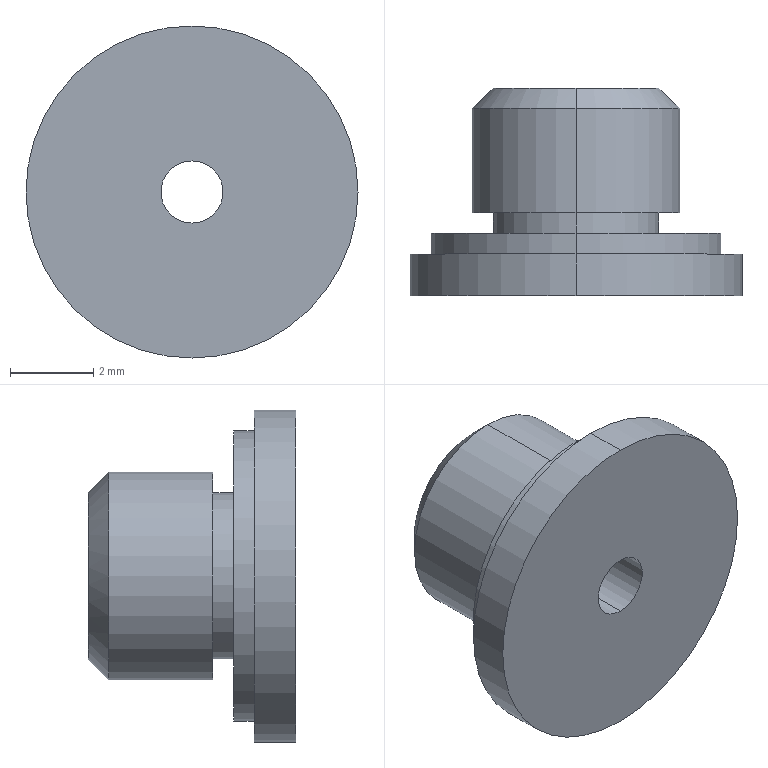Part | SolidWorks | features BaseBody 1 | 1 solid | 17 faces | box 8 x 5 x 8 mm | volume 124.094 mm3 | cylinder 10 | plane 5 | cone 2 | commonest cylinder face diameters 1.5 x2 4 x2 5 x2 7 x2 8 x2
STEP:
#1=CARTESIAN_POINT('',(0.,14.,0.75));
#2=VERTEX_POINT('',#1);
#3=CARTESIAN_POINT('',(0.,14.,-0.75));
#4=VERTEX_POINT('',#3);
#5=CARTESIAN_POINT('',(0.,14.,0.));
#6=DIRECTION('',(0.,-1.,0.));
#7=DIRECTION('',(0.,0.,-1.));
#8=AXIS2_PLACEMENT_3D('',#5,#6,#7);
#9=CIRCLE('',#8,0.75);
#10=EDGE_CURVE('',#2,#4,#9,.T.);
#11=ORIENTED_EDGE('',*,*,#10,.F.);
#12=CARTESIAN_POINT('',(0.,9.,0.75));
#13=VERTEX_POINT('',#12);
#14=CARTESIAN_POINT('',(0.,11.5,0.75));
#15=DIRECTION('',(0.,-1.,0.));
#16=VECTOR('',#15,1000.);
#17=LINE('',#14,#16);
#18=EDGE_CURVE('',#2,#13,#17,.T.);
#19=ORIENTED_EDGE('',*,*,#18,.T.);
#20=CARTESIAN_POINT('',(0.,9.,-0.75));
#21=VERTEX_POINT('',#20);
#22=CARTESIAN_POINT('',(0.,9.,0.));
#23=DIRECTION('',(0.,1.,0.));
#24=DIRECTION('',(0.,0.,-1.));
#25=AXIS2_PLACEMENT_3D('',#22,#23,#24);
#26=CIRCLE('',#25,0.75);
#27=EDGE_CURVE('',#21,#13,#26,.T.);
#28=ORIENTED_EDGE('',*,*,#27,.F.);
#29=CARTESIAN_POINT('',(0.,11.5,-0.75));
#30=DIRECTION('',(0.,-1.,0.));
#31=VECTOR('',#30,1000.);
#32=LINE('',#29,#31);
#33=EDGE_CURVE('',#4,#21,#32,.T.);
#34=ORIENTED_EDGE('',*,*,#33,.F.);
#35=EDGE_LOOP('',(#11,#19,#28,#34));
#36=FACE_OUTER_BOUND('',#35,.T.);
#37=CARTESIAN_POINT('',(0.,11.5,0.));
#38=DIRECTION('',(0.,-1.,0.));
#39=DIRECTION('',(0.,0.,-1.));
#40=AXIS2_PLACEMENT_3D('',#37,#38,#39);
#41=CYLINDRICAL_SURFACE('',#40,0.75);
#42=ADVANCED_FACE('',(#36),#41,.F.);
#43=CARTESIAN_POINT('',(0.,10.,-4.));
#44=VERTEX_POINT('',#43);
#45=CARTESIAN_POINT('',(0.,10.,4.));
#46=VERTEX_POINT('',#45);
#47=CARTESIAN_POINT('',(0.,10.,0.));
#48=DIRECTION('',(0.,-1.,0.));
#49=DIRECTION('',(0.,0.,-1.));
#50=AXIS2_PLACEMENT_3D('',#47,#48,#49);
#51=CIRCLE('',#50,4.);
#52=EDGE_CURVE('',#44,#46,#51,.T.);
#53=ORIENTED_EDGE('',*,*,#52,.T.);
#54=CARTESIAN_POINT('',(0.,9.,4.));
#55=VERTEX_POINT('',#54);
#56=CARTESIAN_POINT('',(0.,9.5,4.));
#57=DIRECTION('',(0.,-1.,0.));
#58=VECTOR('',#57,1000.);
#59=LINE('',#56,#58);
#60=EDGE_CURVE('',#46,#55,#59,.T.);
#61=ORIENTED_EDGE('',*,*,#60,.T.);
#62=CARTESIAN_POINT('',(0.,9.,-4.));
#63=VERTEX_POINT('',#62);
#64=CARTESIAN_POINT('',(0.,9.,0.));
#65=DIRECTION('',(0.,-1.,0.));
#66=DIRECTION('',(0.,0.,-1.));
#67=AXIS2_PLACEMENT_3D('',#64,#65,#66);
#68=CIRCLE('',#67,4.);
#69=EDGE_CURVE('',#63,#55,#68,.T.);
#70=ORIENTED_EDGE('',*,*,#69,.F.);
#71=CARTESIAN_POINT('',(0.,9.5,-4.));
#72=DIRECTION('',(0.,-1.,0.));
#73=VECTOR('',#72,1000.);
#74=LINE('',#71,#73);
#75=EDGE_CURVE('',#44,#63,#74,.T.);
#76=ORIENTED_EDGE('',*,*,#75,.F.);
#77=EDGE_LOOP('',(#53,#61,#70,#76));
#78=FACE_OUTER_BOUND('',#77,.T.);
#79=CARTESIAN_POINT('',(0.,9.5,0.));
#80=DIRECTION('',(0.,-1.,0.));
#81=DIRECTION('',(0.,0.,-1.));
#82=AXIS2_PLACEMENT_3D('',#79,#80,#81);
#83=CYLINDRICAL_SURFACE('',#82,4.);
#84=ADVANCED_FACE('',(#78),#83,.T.);
#85=CARTESIAN_POINT('',(0.,14.,2.009));
#86=VERTEX_POINT('',#85);
#87=CARTESIAN_POINT('',(0.,14.,-2.009));
#88=VERTEX_POINT('',#87);
#89=CARTESIAN_POINT('',(0.,14.,0.));
#90=DIRECTION('',(0.,1.,0.));
#91=DIRECTION('',(0.,0.,-1.));
#92=AXIS2_PLACEMENT_3D('',#89,#90,#91);
#93=CIRCLE('',#92,2.009);
#94=EDGE_CURVE('',#86,#88,#93,.T.);
#95=ORIENTED_EDGE('',*,*,#94,.F.);
#96=CARTESIAN_POINT('',(0.,13.509,2.5));
#97=VERTEX_POINT('',#96);
#98=CARTESIAN_POINT('',(0.,13.51,2.5));
#99=DIRECTION('',(0.,-0.7071,0.7071));
#100=VECTOR('',#99,1000.);
#101=LINE('',#98,#100);
#102=EDGE_CURVE('',#86,#97,#101,.T.);
#103=ORIENTED_EDGE('',*,*,#102,.T.);
#104=CARTESIAN_POINT('',(0.,13.509,-2.5));
#105=VERTEX_POINT('',#104);
#106=CARTESIAN_POINT('',(0.,13.509,0.));
#107=DIRECTION('',(0.,1.,0.));
#108=DIRECTION('',(1.,0.,0.));
#109=AXIS2_PLACEMENT_3D('',#106,#107,#108);
#110=CIRCLE('',#109,2.5);
#111=EDGE_CURVE('',#97,#105,#110,.T.);
#112=ORIENTED_EDGE('',*,*,#111,.T.);
#113=CARTESIAN_POINT('',(0.,13.51,-2.5));
#114=DIRECTION('',(0.,-0.7071,-0.7071));
#115=VECTOR('',#114,1000.);
#116=LINE('',#113,#115);
#117=EDGE_CURVE('',#88,#105,#116,.T.);
#118=ORIENTED_EDGE('',*,*,#117,.F.);
#119=EDGE_LOOP('',(#95,#103,#112,#118));
#120=FACE_OUTER_BOUND('',#119,.T.);
#121=CARTESIAN_POINT('',(0.,13.51,0.));
#122=DIRECTION('',(0.,-1.,0.));
#123=DIRECTION('',(0.,0.,-1.));
#124=AXIS2_PLACEMENT_3D('',#121,#122,#123);
#125=CONICAL_SURFACE('',#124,2.5,0.7854);
#126=ADVANCED_FACE('',(#120),#125,.T.);
#127=CARTESIAN_POINT('',(0.,10.5,-3.5));
#128=VERTEX_POINT('',#127);
#129=CARTESIAN_POINT('',(0.,10.5,3.5));
#130=VERTEX_POINT('',#129);
#131=CARTESIAN_POINT('',(0.,10.5,0.));
#132=DIRECTION('',(0.,-1.,0.));
#133=DIRECTION('',(0.,0.,-1.));
#134=AXIS2_PLACEMENT_3D('',#131,#132,#133);
#135=CIRCLE('',#134,3.5);
#136=EDGE_CURVE('',#128,#130,#135,.T.);
#137=ORIENTED_EDGE('',*,*,#136,.T.);
#138=CARTESIAN_POINT('',(0.,10.,3.5));
#139=VERTEX_POINT('',#138);
#140=CARTESIAN_POINT('',(0.,10.25,3.5));
#141=DIRECTION('',(0.,-1.,0.));
#142=VECTOR('',#141,1000.);
#143=LINE('',#140,#142);
#144=EDGE_CURVE('',#130,#139,#143,.T.);
#145=ORIENTED_EDGE('',*,*,#144,.T.);
#146=CARTESIAN_POINT('',(0.,10.,-3.5));
#147=VERTEX_POINT('',#146);
#148=CARTESIAN_POINT('',(0.,10.,0.));
#149=DIRECTION('',(0.,-1.,0.));
#150=DIRECTION('',(0.,0.,-1.));
#151=AXIS2_PLACEMENT_3D('',#148,#149,#150);
#152=CIRCLE('',#151,3.5);
#153=EDGE_CURVE('',#147,#139,#152,.T.);
#154=ORIENTED_EDGE('',*,*,#153,.F.);
#155=CARTESIAN_POINT('',(0.,10.25,-3.5));
#156=DIRECTION('',(0.,-1.,0.));
#157=VECTOR('',#156,1000.);
#158=LINE('',#155,#157);
#159=EDGE_CURVE('',#128,#147,#158,.T.);
#160=ORIENTED_EDGE('',*,*,#159,.F.);
#161=EDGE_LOOP('',(#137,#145,#154,#160));
#162=FACE_OUTER_BOUND('',#161,.T.);
#163=CARTESIAN_POINT('',(0.,10.25,0.));
#164=DIRECTION('',(0.,-1.,0.));
#165=DIRECTION('',(0.,0.,-1.));
#166=AXIS2_PLACEMENT_3D('',#163,#164,#165);
#167=CYLINDRICAL_SURFACE('',#166,3.5);
#168=ADVANCED_FACE('',(#162),#167,.T.);
#169=ORIENTED_EDGE('',*,*,#111,.F.);
#170=CARTESIAN_POINT('',(0.,11.,2.5));
#171=VERTEX_POINT('',#170);
#172=CARTESIAN_POINT('',(0.,12.255,2.5));
#173=DIRECTION('',(0.,-1.,0.));
#174=VECTOR('',#173,1000.);
#175=LINE('',#172,#174);
#176=EDGE_CURVE('',#97,#171,#175,.T.);
#177=ORIENTED_EDGE('',*,*,#176,.T.);
#178=CARTESIAN_POINT('',(0.,11.,-2.5));
#179=VERTEX_POINT('',#178);
#180=CARTESIAN_POINT('',(0.,11.,0.));
#181=DIRECTION('',(0.,1.,0.));
#182=DIRECTION('',(0.,0.,-1.));
#183=AXIS2_PLACEMENT_3D('',#180,#181,#182);
#184=CIRCLE('',#183,2.5);
#185=EDGE_CURVE('',#171,#179,#184,.T.);
#186=ORIENTED_EDGE('',*,*,#185,.T.);
#187=CARTESIAN_POINT('',(0.,12.255,-2.5));
#188=DIRECTION('',(0.,-1.,0.));
#189=VECTOR('',#188,1000.);
#190=LINE('',#187,#189);
#191=EDGE_CURVE('',#105,#179,#190,.T.);
#192=ORIENTED_EDGE('',*,*,#191,.F.);
#193=EDGE_LOOP('',(#169,#177,#186,#192));
#194=FACE_OUTER_BOUND('',#193,.T.);
#195=CARTESIAN_POINT('',(0.,12.255,0.));
#196=DIRECTION('',(0.,-1.,0.));
#197=DIRECTION('',(0.,0.,-1.));
#198=AXIS2_PLACEMENT_3D('',#195,#196,#197);
#199=CYLINDRICAL_SURFACE('',#198,2.5);
#200=ADVANCED_FACE('',(#194),#199,.T.);
#201=CARTESIAN_POINT('',(0.,11.,2.));
#202=VERTEX_POINT('',#201);
#203=CARTESIAN_POINT('',(0.,11.,-2.));
#204=VERTEX_POINT('',#203);
#205=CARTESIAN_POINT('',(0.,11.,0.));
#206=DIRECTION('',(0.,1.,0.));
#207=DIRECTION('',(0.,0.,-1.));
#208=AXIS2_PLACEMENT_3D('',#205,#206,#207);
#209=CIRCLE('',#208,2.);
#210=EDGE_CURVE('',#202,#204,#209,.T.);
#211=ORIENTED_EDGE('',*,*,#210,.F.);
#212=CARTESIAN_POINT('',(0.,10.5,2.));
#213=VERTEX_POINT('',#212);
#214=CARTESIAN_POINT('',(0.,10.75,2.));
#215=DIRECTION('',(0.,-1.,0.));
#216=VECTOR('',#215,1000.);
#217=LINE('',#214,#216);
#218=EDGE_CURVE('',#202,#213,#217,.T.);
#219=ORIENTED_EDGE('',*,*,#218,.T.);
#220=CARTESIAN_POINT('',(0.,10.5,-2.));
#221=VERTEX_POINT('',#220);
#222=CARTESIAN_POINT('',(0.,10.5,0.));
#223=DIRECTION('',(0.,-1.,0.));
#224=DIRECTION('',(0.,0.,-1.));
#225=AXIS2_PLACEMENT_3D('',#222,#223,#224);
#226=CIRCLE('',#225,2.);
#227=EDGE_CURVE('',#221,#213,#226,.T.);
#228=ORIENTED_EDGE('',*,*,#227,.F.);
#229=CARTESIAN_POINT('',(0.,10.75,-2.));
#230=DIRECTION('',(0.,-1.,0.));
#231=VECTOR('',#230,1000.);
#232=LINE('',#229,#231);
#233=EDGE_CURVE('',#204,#221,#232,.T.);
#234=ORIENTED_EDGE('',*,*,#233,.F.);
#235=EDGE_LOOP('',(#211,#219,#228,#234));
#236=FACE_OUTER_BOUND('',#235,.T.);
#237=CARTESIAN_POINT('',(0.,10.75,0.));
#238=DIRECTION('',(0.,-1.,0.));
#239=DIRECTION('',(0.,0.,-1.));
#240=AXIS2_PLACEMENT_3D('',#237,#238,#239);
#241=CYLINDRICAL_SURFACE('',#240,2.);
#242=ADVANCED_FACE('',(#236),#241,.T.);
#243=CARTESIAN_POINT('',(0.,11.,0.));
#244=DIRECTION('',(0.,1.,0.));
#245=DIRECTION('',(0.,0.,-1.));
#246=AXIS2_PLACEMENT_3D('',#243,#244,#245);
#247=CIRCLE('',#246,2.);
#248=EDGE_CURVE('',#204,#202,#247,.T.);
#249=ORIENTED_EDGE('',*,*,#248,.T.);
#250=ORIENTED_EDGE('',*,*,#210,.T.);
#251=EDGE_LOOP('',(#249,#250));
#252=FACE_BOUND('',#251,.T.);
#253=CARTESIAN_POINT('',(0.,11.,0.));
#254=DIRECTION('',(0.,1.,0.));
#255=DIRECTION('',(0.,0.,-1.));
#256=AXIS2_PLACEMENT_3D('',#253,#254,#255);
#257=CIRCLE('',#256,2.5);
#258=EDGE_CURVE('',#179,#171,#257,.T.);
#259=ORIENTED_EDGE('',*,*,#258,.F.);
#260=ORIENTED_EDGE('',*,*,#185,.F.);
#261=EDGE_LOOP('',(#259,#260));
#262=FACE_OUTER_BOUND('',#261,.T.);
#263=CARTESIAN_POINT('',(2.25,11.,0.));
#264=DIRECTION('',(0.,-1.,0.));
#265=DIRECTION('',(0.,0.,-1.));
#266=AXIS2_PLACEMENT_3D('',#263,#264,#265);
#267=PLANE('',#266);
#268=ADVANCED_FACE('',(#252,#262),#267,.T.);
#269=ORIENTED_EDGE('',*,*,#227,.T.);
#270=CARTESIAN_POINT('',(0.,10.5,0.));
#271=DIRECTION('',(0.,-1.,0.));
#272=DIRECTION('',(0.,0.,-1.));
#273=AXIS2_PLACEMENT_3D('',#270,#271,#272);
#274=CIRCLE('',#273,2.);
#275=EDGE_CURVE('',#213,#221,#274,.T.);
#276=ORIENTED_EDGE('',*,*,#275,.T.);
#277=EDGE_LOOP('',(#269,#276));
#278=FACE_BOUND('',#277,.T.);
#279=ORIENTED_EDGE('',*,*,#136,.F.);
#280=CARTESIAN_POINT('',(0.,10.5,0.));
#281=DIRECTION('',(0.,-1.,0.));
#282=DIRECTION('',(0.,0.,-1.));
#283=AXIS2_PLACEMENT_3D('',#280,#281,#282);
#284=CIRCLE('',#283,3.5);
#285=EDGE_CURVE('',#130,#128,#284,.T.);
#286=ORIENTED_EDGE('',*,*,#285,.F.);
#287=EDGE_LOOP('',(#279,#286));
#288=FACE_OUTER_BOUND('',#287,.T.);
#289=CARTESIAN_POINT('',(2.75,10.5,0.));
#290=DIRECTION('',(0.,1.,0.));
#291=DIRECTION('',(1.,0.,0.));
#292=AXIS2_PLACEMENT_3D('',#289,#290,#291);
#293=PLANE('',#292);
#294=ADVANCED_FACE('',(#278,#288),#293,.T.);
#295=ORIENTED_EDGE('',*,*,#153,.T.);
#296=CARTESIAN_POINT('',(0.,10.,0.));
#297=DIRECTION('',(0.,-1.,0.));
#298=DIRECTION('',(0.,0.,-1.));
#299=AXIS2_PLACEMENT_3D('',#296,#297,#298);
#300=CIRCLE('',#299,3.5);
#301=EDGE_CURVE('',#139,#147,#300,.T.);
#302=ORIENTED_EDGE('',*,*,#301,.T.);
#303=EDGE_LOOP('',(#295,#302));
#304=FACE_BOUND('',#303,.T.);
#305=ORIENTED_EDGE('',*,*,#52,.F.);
#306=CARTESIAN_POINT('',(0.,10.,0.));
#307=DIRECTION('',(0.,-1.,0.));
#308=DIRECTION('',(0.,0.,-1.));
#309=AXIS2_PLACEMENT_3D('',#306,#307,#308);
#310=CIRCLE('',#309,4.);
#311=EDGE_CURVE('',#46,#44,#310,.T.);
#312=ORIENTED_EDGE('',*,*,#311,.F.);
#313=EDGE_LOOP('',(#305,#312));
#314=FACE_OUTER_BOUND('',#313,.T.);
#315=CARTESIAN_POINT('',(3.75,10.,0.));
#316=DIRECTION('',(0.,1.,0.));
#317=DIRECTION('',(1.,0.,0.));
#318=AXIS2_PLACEMENT_3D('',#315,#316,#317);
#319=PLANE('',#318);
#320=ADVANCED_FACE('',(#304,#314),#319,.T.);
#321=CARTESIAN_POINT('',(0.,14.,0.));
#322=DIRECTION('',(0.,-1.,0.));
#323=DIRECTION('',(0.,0.,-1.));
#324=AXIS2_PLACEMENT_3D('',#321,#322,#323);
#325=CIRCLE('',#324,0.75);
#326=EDGE_CURVE('',#4,#2,#325,.T.);
#327=ORIENTED_EDGE('',*,*,#326,.T.);
#328=ORIENTED_EDGE('',*,*,#10,.T.);
#329=EDGE_LOOP('',(#327,#328));
#330=FACE_BOUND('',#329,.T.);
#331=CARTESIAN_POINT('',(0.,14.,0.));
#332=DIRECTION('',(0.,1.,0.));
#333=DIRECTION('',(0.,0.,-1.));
#334=AXIS2_PLACEMENT_3D('',#331,#332,#333);
#335=CIRCLE('',#334,2.009);
#336=EDGE_CURVE('',#88,#86,#335,.T.);
#337=ORIENTED_EDGE('',*,*,#336,.T.);
#338=ORIENTED_EDGE('',*,*,#94,.T.);
#339=EDGE_LOOP('',(#337,#338));
#340=FACE_OUTER_BOUND('',#339,.T.);
#341=CARTESIAN_POINT('',(1.38,14.,0.));
#342=DIRECTION('',(0.,1.,0.));
#343=DIRECTION('',(1.,0.,0.));
#344=AXIS2_PLACEMENT_3D('',#341,#342,#343);
#345=PLANE('',#344);
#346=ADVANCED_FACE('',(#330,#340),#345,.T.);
#347=ORIENTED_EDGE('',*,*,#27,.T.);
#348=CARTESIAN_POINT('',(0.,9.,0.));
#349=DIRECTION('',(0.,1.,0.));
#350=DIRECTION('',(0.,0.,-1.));
#351=AXIS2_PLACEMENT_3D('',#348,#349,#350);
#352=CIRCLE('',#351,0.75);
#353=EDGE_CURVE('',#13,#21,#352,.T.);
#354=ORIENTED_EDGE('',*,*,#353,.T.);
#355=EDGE_LOOP('',(#347,#354));
#356=FACE_BOUND('',#355,.T.);
#357=ORIENTED_EDGE('',*,*,#69,.T.);
#358=CARTESIAN_POINT('',(0.,9.,0.));
#359=DIRECTION('',(0.,-1.,0.));
#360=DIRECTION('',(0.,0.,-1.));
#361=AXIS2_PLACEMENT_3D('',#358,#359,#360);
#362=CIRCLE('',#361,4.);
#363=EDGE_CURVE('',#55,#63,#362,.T.);
#364=ORIENTED_EDGE('',*,*,#363,.T.);
#365=EDGE_LOOP('',(#357,#364));
#366=FACE_OUTER_BOUND('',#365,.T.);
#367=CARTESIAN_POINT('',(2.375,9.,0.));
#368=DIRECTION('',(0.,-1.,0.));
#369=DIRECTION('',(0.,0.,-1.));
#370=AXIS2_PLACEMENT_3D('',#367,#368,#369);
#371=PLANE('',#370);
#372=ADVANCED_FACE('',(#356,#366),#371,.T.);
#373=ORIENTED_EDGE('',*,*,#218,.F.);
#374=ORIENTED_EDGE('',*,*,#248,.F.);
#375=ORIENTED_EDGE('',*,*,#233,.T.);
#376=ORIENTED_EDGE('',*,*,#275,.F.);
#377=EDGE_LOOP('',(#373,#374,#375,#376));
#378=FACE_OUTER_BOUND('',#377,.T.);
#379=CARTESIAN_POINT('',(0.,10.75,0.));
#380=DIRECTION('',(0.,-1.,0.));
#381=DIRECTION('',(0.,0.,-1.));
#382=AXIS2_PLACEMENT_3D('',#379,#380,#381);
#383=CYLINDRICAL_SURFACE('',#382,2.);
#384=ADVANCED_FACE('',(#378),#383,.T.);
#385=ORIENTED_EDGE('',*,*,#176,.F.);
#386=CARTESIAN_POINT('',(0.,13.509,0.));
#387=DIRECTION('',(0.,1.,0.));
#388=DIRECTION('',(1.,0.,0.));
#389=AXIS2_PLACEMENT_3D('',#386,#387,#388);
#390=CIRCLE('',#389,2.5);
#391=EDGE_CURVE('',#105,#97,#390,.T.);
#392=ORIENTED_EDGE('',*,*,#391,.F.);
#393=ORIENTED_EDGE('',*,*,#191,.T.);
#394=ORIENTED_EDGE('',*,*,#258,.T.);
#395=EDGE_LOOP('',(#385,#392,#393,#394));
#396=FACE_OUTER_BOUND('',#395,.T.);
#397=CARTESIAN_POINT('',(0.,12.255,0.));
#398=DIRECTION('',(0.,-1.,0.));
#399=DIRECTION('',(0.,0.,-1.));
#400=AXIS2_PLACEMENT_3D('',#397,#398,#399);
#401=CYLINDRICAL_SURFACE('',#400,2.5);
#402=ADVANCED_FACE('',(#396),#401,.T.);
#403=ORIENTED_EDGE('',*,*,#144,.F.);
#404=ORIENTED_EDGE('',*,*,#285,.T.);
#405=ORIENTED_EDGE('',*,*,#159,.T.);
#406=ORIENTED_EDGE('',*,*,#301,.F.);
#407=EDGE_LOOP('',(#403,#404,#405,#406));
#408=FACE_OUTER_BOUND('',#407,.T.);
#409=CARTESIAN_POINT('',(0.,10.25,0.));
#410=DIRECTION('',(0.,-1.,0.));
#411=DIRECTION('',(0.,0.,-1.));
#412=AXIS2_PLACEMENT_3D('',#409,#410,#411);
#413=CYLINDRICAL_SURFACE('',#412,3.5);
#414=ADVANCED_FACE('',(#408),#413,.T.);
#415=ORIENTED_EDGE('',*,*,#102,.F.);
#416=ORIENTED_EDGE('',*,*,#336,.F.);
#417=ORIENTED_EDGE('',*,*,#117,.T.);
#418=ORIENTED_EDGE('',*,*,#391,.T.);
#419=EDGE_LOOP('',(#415,#416,#417,#418));
#420=FACE_OUTER_BOUND('',#419,.T.);
#421=CARTESIAN_POINT('',(0.,13.51,0.));
#422=DIRECTION('',(0.,-1.,0.));
#423=DIRECTION('',(0.,0.,-1.));
#424=AXIS2_PLACEMENT_3D('',#421,#422,#423);
#425=CONICAL_SURFACE('',#424,2.5,0.7854);
#426=ADVANCED_FACE('',(#420),#425,.T.);
#427=ORIENTED_EDGE('',*,*,#60,.F.);
#428=ORIENTED_EDGE('',*,*,#311,.T.);
#429=ORIENTED_EDGE('',*,*,#75,.T.);
#430=ORIENTED_EDGE('',*,*,#363,.F.);
#431=EDGE_LOOP('',(#427,#428,#429,#430));
#432=FACE_OUTER_BOUND('',#431,.T.);
#433=CARTESIAN_POINT('',(0.,9.5,0.));
#434=DIRECTION('',(0.,-1.,0.));
#435=DIRECTION('',(0.,0.,-1.));
#436=AXIS2_PLACEMENT_3D('',#433,#434,#435);
#437=CYLINDRICAL_SURFACE('',#436,4.);
#438=ADVANCED_FACE('',(#432),#437,.T.);
#439=ORIENTED_EDGE('',*,*,#18,.F.);
#440=ORIENTED_EDGE('',*,*,#326,.F.);
#441=ORIENTED_EDGE('',*,*,#33,.T.);
#442=ORIENTED_EDGE('',*,*,#353,.F.);
#443=EDGE_LOOP('',(#439,#440,#441,#442));
#444=FACE_OUTER_BOUND('',#443,.T.);
#445=CARTESIAN_POINT('',(0.,11.5,0.));
#446=DIRECTION('',(0.,-1.,0.));
#447=DIRECTION('',(0.,0.,-1.));
#448=AXIS2_PLACEMENT_3D('',#445,#446,#447);
#449=CYLINDRICAL_SURFACE('',#448,0.75);
#450=ADVANCED_FACE('',(#444),#449,.F.);
#451=CLOSED_SHELL('',(#42,#84,#126,#168,#200,#242,#268,#294,#320,#346,#372,#384,#402,#414,#426,#438,#450));
#452=MANIFOLD_SOLID_BREP('',#451);
#453=CARTESIAN_POINT('',(0.,0.,0.));
#454=DIRECTION('',(0.,0.,1.));
#455=DIRECTION('',(1.,0.,0.));
#456=AXIS2_PLACEMENT_3D('',#453,#454,#455);
#457=(LENGTH_UNIT()NAMED_UNIT(*)SI_UNIT(.MILLI.,.METRE.));
#458=UNCERTAINTY_MEASURE_WITH_UNIT(LENGTH_MEASURE(0.00001),#457,'','');
#459=(NAMED_UNIT(*)PLANE_ANGLE_UNIT()SI_UNIT($,.RADIAN.));
#460=(NAMED_UNIT(*)SI_UNIT($,.STERADIAN.)SOLID_ANGLE_UNIT());
#461=(GEOMETRIC_REPRESENTATION_CONTEXT(3)GLOBAL_UNCERTAINTY_ASSIGNED_CONTEXT((#458))GLOBAL_UNIT_ASSIGNED_CONTEXT((#457,#459,#460))REPRESENTATION_CONTEXT('',''));
#462=ADVANCED_BREP_SHAPE_REPRESENTATION('',(#452,#456),#461);